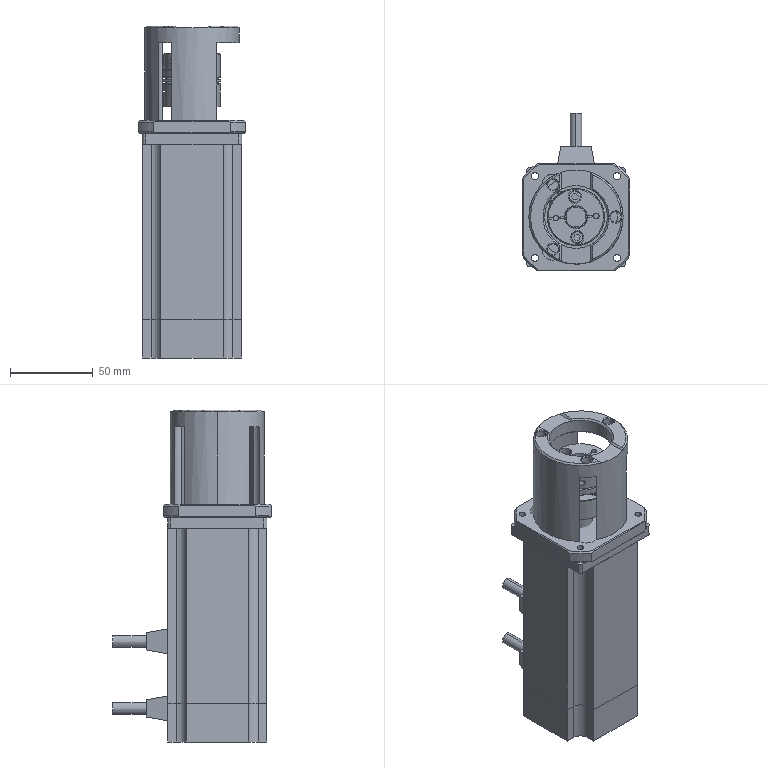Part | STEP file | Copy of 400W motor assembly (60 motor base)^K50A-1H20-S(formula driven)-L300-motor left- | 10 solids | 408 faces | box 65 x 95.5 x 200.5 mm | volume 502014 mm3 | plane 175 | cylinder 166 | cone 67 | commonest cylinder face diameters 7 x32 3.3 x21 8 x19 3.1 x14 12 x12 4.2 x8